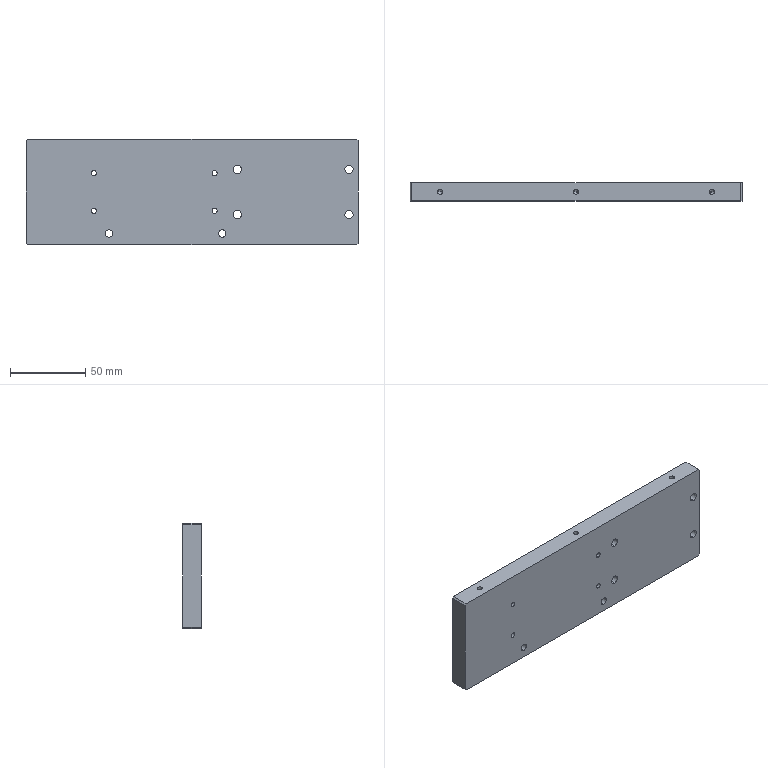Part | NX | features BREP 1 | 1 solid | 66 faces | box 220 x 12 x 70 mm | volume 180436 mm3 | cylinder 40 | plane 14 | cone 12 | commonest cylinder face diameters 3.3 x20 5.5 x8 11 x8 5 x4